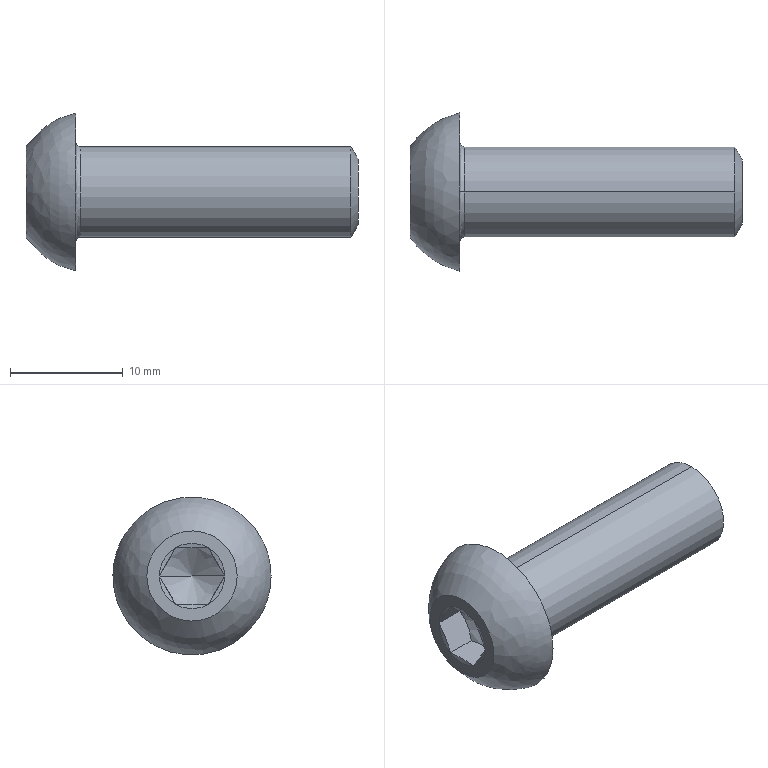Part | SolidWorks | features BaseBody 1 | 1 solid | 24 faces | box 29.4 x 14 x 14 mm | volume 1672 mm3 | cone 10 | plane 9 | spline 3 | cylinder 2 | commonest cylinder face diameters 8 x2
STEP:
#1=CARTESIAN_POINT('',(-24.6,0.,-4.));
#2=VERTEX_POINT('',#1);
#3=CARTESIAN_POINT('',(-24.6,0.,4.));
#4=VERTEX_POINT('',#3);
#5=CARTESIAN_POINT('',(-24.6,0.,0.));
#6=DIRECTION('',(1.,0.,0.));
#7=DIRECTION('',(0.,0.,1.));
#8=AXIS2_PLACEMENT_3D('',#5,#6,#7);
#9=CIRCLE('',#8,4.);
#10=EDGE_CURVE('',#2,#4,#9,.T.);
#11=ORIENTED_EDGE('',*,*,#10,.F.);
#12=CARTESIAN_POINT('',(-25.,0.,-4.4));
#13=VERTEX_POINT('',#12);
#14=CARTESIAN_POINT('',(-24.6,0.,-4.4));
#15=DIRECTION('',(0.,-1.,0.));
#16=DIRECTION('',(0.,0.,-1.));
#17=AXIS2_PLACEMENT_3D('',#14,#15,#16);
#18=CIRCLE('',#17,0.4);
#19=EDGE_CURVE('',#2,#13,#18,.T.);
#20=ORIENTED_EDGE('',*,*,#19,.T.);
#21=CARTESIAN_POINT('',(-25.,0.,4.4));
#22=VERTEX_POINT('',#21);
#23=CARTESIAN_POINT('',(-25.,0.,4.4));
#24=CARTESIAN_POINT('',(-25.,0.2798,4.4));
#25=CARTESIAN_POINT('',(-25.,0.6922,4.361));
#26=CARTESIAN_POINT('',(-25.,1.16,4.249));
#27=CARTESIAN_POINT('',(-25.,1.391,4.176));
#28=CARTESIAN_POINT('',(-25.,1.506,4.135));
#29=CARTESIAN_POINT('',(-25.,1.555,4.116));
#30=CARTESIAN_POINT('',(-25.,1.587,4.104));
#31=CARTESIAN_POINT('',(-25.,1.602,4.098));
#32=CARTESIAN_POINT('',(-25.,1.758,4.036));
#33=CARTESIAN_POINT('',(-25.,1.96,3.944));
#34=CARTESIAN_POINT('',(-25.,2.155,3.837));
#35=CARTESIAN_POINT('',(-25.,2.283,3.762));
#36=CARTESIAN_POINT('',(-25.,2.344,3.724));
#37=CARTESIAN_POINT('',(-25.,2.662,3.516));
#38=CARTESIAN_POINT('',(-25.,2.896,3.326));
#39=CARTESIAN_POINT('',(-25.,3.219,3.004));
#40=CARTESIAN_POINT('',(-25.,3.371,2.835));
#41=CARTESIAN_POINT('',(-25.,3.509,2.656));
#42=CARTESIAN_POINT('',(-25.,3.598,2.533));
#43=CARTESIAN_POINT('',(-25.,3.642,2.47));
#44=CARTESIAN_POINT('',(-25.,3.764,2.283));
#45=CARTESIAN_POINT('',(-25.,3.876,2.091));
#46=CARTESIAN_POINT('',(-25.,3.99,1.858));
#47=CARTESIAN_POINT('',(-25.,4.034,1.757));
#48=CARTESIAN_POINT('',(-25.,4.063,1.688));
#49=CARTESIAN_POINT('',(-25.,4.078,1.652));
#50=CARTESIAN_POINT('',(-25.,4.297,1.099));
#51=CARTESIAN_POINT('',(-25.,4.4,0.5599));
#52=CARTESIAN_POINT('',(-25.,4.4,-0.2799));
#53=CARTESIAN_POINT('',(-25.,4.361,-0.6923));
#54=CARTESIAN_POINT('',(-25.,4.249,-1.16));
#55=CARTESIAN_POINT('',(-25.,4.176,-1.391));
#56=CARTESIAN_POINT('',(-25.,4.135,-1.506));
#57=CARTESIAN_POINT('',(-25.,4.116,-1.555));
#58=CARTESIAN_POINT('',(-25.,4.104,-1.587));
#59=CARTESIAN_POINT('',(-25.,4.098,-1.602));
#60=CARTESIAN_POINT('',(-25.,4.036,-1.758));
#61=CARTESIAN_POINT('',(-25.,3.944,-1.96));
#62=CARTESIAN_POINT('',(-25.,3.837,-2.155));
#63=CARTESIAN_POINT('',(-25.,3.762,-2.283));
#64=CARTESIAN_POINT('',(-25.,3.724,-2.344));
#65=CARTESIAN_POINT('',(-25.,3.516,-2.662));
#66=CARTESIAN_POINT('',(-25.,3.326,-2.896));
#67=CARTESIAN_POINT('',(-25.,3.004,-3.219));
#68=CARTESIAN_POINT('',(-25.,2.835,-3.371));
#69=CARTESIAN_POINT('',(-25.,2.656,-3.509));
#70=CARTESIAN_POINT('',(-25.,2.533,-3.598));
#71=CARTESIAN_POINT('',(-25.,2.47,-3.642));
#72=CARTESIAN_POINT('',(-25.,2.283,-3.764));
#73=CARTESIAN_POINT('',(-25.,2.091,-3.876));
#74=CARTESIAN_POINT('',(-25.,1.858,-3.99));
#75=CARTESIAN_POINT('',(-25.,1.757,-4.034));
#76=CARTESIAN_POINT('',(-25.,1.688,-4.063));
#77=CARTESIAN_POINT('',(-25.,1.652,-4.078));
#78=CARTESIAN_POINT('',(-25.,1.099,-4.297));
#79=CARTESIAN_POINT('',(-25.,0.5593,-4.4));
#80=CARTESIAN_POINT('',(-25.,0.,-4.4));
#81=B_SPLINE_CURVE_WITH_KNOTS('',3,(#23,#24,#25,#26,#27,#28,#29,#30,#31,#32,#33,#34,#35,#36,#37,#38,#39,#40,#41,#42,#43,#44,#45,#46,#47,#48,#49,#50,#51,#52,#53,#54,#55,#56,#57,#58,#59,#60,#61,#62,#63,#64,#65,#66,#67,#68,#69,#70,#71,#72,#73,#74,#75,#76,#77,#78,#79,#80),.UNSPECIFIED.,.F.,.F.,(4,1,1,1,1,2,2,1,2,2,2,1,2,2,1,1,2,2,2,1,1,1,1,2,2,1,2,2,2,1,2,2,1,1,2,2,4),(0.,0.0625,0.09375,0.1094,0.1172,0.1211,0.125,0.1562,0.1719,0.1875,0.25,0.2812,0.2969,0.3125,0.3437,0.3594,0.3672,0.375,0.5,0.5625,0.5937,0.6094,0.6172,0.6211,0.625,0.6562,0.6719,0.6875,0.75,0.7812,0.7969,0.8125,0.8437,0.8594,0.8672,0.875,1.),.UNSPECIFIED.);
#82=EDGE_CURVE('',#22,#13,#81,.T.);
#83=ORIENTED_EDGE('',*,*,#82,.F.);
#84=CARTESIAN_POINT('',(-24.6,0.,4.4));
#85=DIRECTION('',(0.,1.,0.));
#86=DIRECTION('',(0.,0.,1.));
#87=AXIS2_PLACEMENT_3D('',#84,#85,#86);
#88=CIRCLE('',#87,0.4);
#89=EDGE_CURVE('',#4,#22,#88,.T.);
#90=ORIENTED_EDGE('',*,*,#89,.F.);
#91=EDGE_LOOP('',(#11,#20,#83,#90));
#92=FACE_OUTER_BOUND('',#91,.T.);
#93=CARTESIAN_POINT('',(-24.6,0.,4.));
#94=CARTESIAN_POINT('',(-24.6,8.,4.));
#95=CARTESIAN_POINT('',(-24.6,8.,-4.));
#96=CARTESIAN_POINT('',(-24.6,0.,-4.));
#97=CARTESIAN_POINT('',(-24.834,0.,4.));
#98=CARTESIAN_POINT('',(-24.834,8.,4.));
#99=CARTESIAN_POINT('',(-24.834,8.,-4.));
#100=CARTESIAN_POINT('',(-24.834,0.,-4.));
#101=CARTESIAN_POINT('',(-25.,0.,4.166));
#102=CARTESIAN_POINT('',(-25.,8.331,4.166));
#103=CARTESIAN_POINT('',(-25.,8.331,-4.166));
#104=CARTESIAN_POINT('',(-25.,0.,-4.166));
#105=CARTESIAN_POINT('',(-25.,0.,4.4));
#106=CARTESIAN_POINT('',(-25.,8.8,4.4));
#107=CARTESIAN_POINT('',(-25.,8.8,-4.4));
#108=CARTESIAN_POINT('',(-25.,0.,-4.4));
#109=(BOUNDED_SURFACE()B_SPLINE_SURFACE(3,3,((#93,#94,#95,#96),(#97,#98,#99,#100),(#101,#102,#103,#104),(#105,#106,#107,#108)),.UNSPECIFIED.,.F.,.F.,.F.)B_SPLINE_SURFACE_WITH_KNOTS((4,4),(4,4),(0.,1.),(0.,1.),.UNSPECIFIED.)GEOMETRIC_REPRESENTATION_ITEM()RATIONAL_B_SPLINE_SURFACE(((1.,0.3333,0.3333,1.),(0.8047,0.2682,0.2682,0.8047),(0.8047,0.2682,0.2682,0.8047),(1.,0.3333,0.3333,1.)))REPRESENTATION_ITEM('')SURFACE());
#110=ADVANCED_FACE('',(#92),#109,.F.);
#111=CARTESIAN_POINT('',(-0.625,0.,4.));
#112=VERTEX_POINT('',#111);
#113=CARTESIAN_POINT('',(-0.625,0.,-4.));
#114=VERTEX_POINT('',#113);
#115=CARTESIAN_POINT('',(-0.625,0.,0.));
#116=DIRECTION('',(-1.,0.,0.));
#117=DIRECTION('',(0.,0.,1.));
#118=AXIS2_PLACEMENT_3D('',#115,#116,#117);
#119=CIRCLE('',#118,4.);
#120=EDGE_CURVE('',#112,#114,#119,.T.);
#121=ORIENTED_EDGE('',*,*,#120,.T.);
#122=CARTESIAN_POINT('',(-29.4,0.,-4.));
#123=DIRECTION('',(-1.,0.,0.));
#124=VECTOR('',#123,1000.);
#125=LINE('',#122,#124);
#126=EDGE_CURVE('',#114,#2,#125,.T.);
#127=ORIENTED_EDGE('',*,*,#126,.T.);
#128=ORIENTED_EDGE('',*,*,#10,.T.);
#129=CARTESIAN_POINT('',(-29.4,0.,4.));
#130=DIRECTION('',(-1.,0.,0.));
#131=VECTOR('',#130,1000.);
#132=LINE('',#129,#131);
#133=EDGE_CURVE('',#112,#4,#132,.T.);
#134=ORIENTED_EDGE('',*,*,#133,.F.);
#135=EDGE_LOOP('',(#121,#127,#128,#134));
#136=FACE_OUTER_BOUND('',#135,.T.);
#137=CARTESIAN_POINT('',(-29.4,0.,0.));
#138=DIRECTION('',(-1.,0.,0.));
#139=DIRECTION('',(0.,0.,1.));
#140=AXIS2_PLACEMENT_3D('',#137,#138,#139);
#141=CYLINDRICAL_SURFACE('',#140,4.);
#142=ADVANCED_FACE('',(#136),#141,.T.);
#143=CARTESIAN_POINT('',(0.,0.,2.917));
#144=VERTEX_POINT('',#143);
#145=CARTESIAN_POINT('',(0.,0.,-2.917));
#146=VERTEX_POINT('',#145);
#147=CARTESIAN_POINT('',(0.,0.,0.));
#148=DIRECTION('',(-1.,0.,0.));
#149=DIRECTION('',(0.,0.,1.));
#150=AXIS2_PLACEMENT_3D('',#147,#148,#149);
#151=CIRCLE('',#150,2.917);
#152=EDGE_CURVE('',#144,#146,#151,.T.);
#153=ORIENTED_EDGE('',*,*,#152,.T.);
#154=CARTESIAN_POINT('',(-0.625,0.,-4.));
#155=DIRECTION('',(-0.5,0.,-0.866));
#156=VECTOR('',#155,1000.);
#157=LINE('',#154,#156);
#158=EDGE_CURVE('',#146,#114,#157,.T.);
#159=ORIENTED_EDGE('',*,*,#158,.T.);
#160=ORIENTED_EDGE('',*,*,#120,.F.);
#161=CARTESIAN_POINT('',(-0.625,0.,4.));
#162=DIRECTION('',(-0.5,0.,0.866));
#163=VECTOR('',#162,1000.);
#164=LINE('',#161,#163);
#165=EDGE_CURVE('',#144,#112,#164,.T.);
#166=ORIENTED_EDGE('',*,*,#165,.F.);
#167=EDGE_LOOP('',(#153,#159,#160,#166));
#168=FACE_OUTER_BOUND('',#167,.T.);
#169=CARTESIAN_POINT('',(-0.625,0.,0.));
#170=DIRECTION('',(-1.,0.,0.));
#171=DIRECTION('',(0.,0.,1.));
#172=AXIS2_PLACEMENT_3D('',#169,#170,#171);
#173=CONICAL_SURFACE('',#172,4.,1.047);
#174=ADVANCED_FACE('',(#168),#173,.T.);
#175=CARTESIAN_POINT('',(-25.,0.,0.));
#176=VERTEX_POINT('',#175);
#177=CARTESIAN_POINT('',(-26.8,-2.887,0.));
#178=VERTEX_POINT('',#177);
#179=CARTESIAN_POINT('',(-26.811,-2.904,0.));
#180=DIRECTION('',(-0.5291,-0.8486,0.));
#181=VECTOR('',#180,1000.);
#182=LINE('',#179,#181);
#183=EDGE_CURVE('',#176,#178,#182,.T.);
#184=ORIENTED_EDGE('',*,*,#183,.F.);
#185=CARTESIAN_POINT('',(-26.8,2.887,-0.000000014));
#186=VERTEX_POINT('',#185);
#187=CARTESIAN_POINT('',(-26.811,2.904,0.));
#188=DIRECTION('',(-0.5291,0.8486,0.));
#189=VECTOR('',#188,1000.);
#190=LINE('',#187,#189);
#191=EDGE_CURVE('',#176,#186,#190,.T.);
#192=ORIENTED_EDGE('',*,*,#191,.T.);
#193=CARTESIAN_POINT('',(-26.8,1.443,-2.5));
#194=VERTEX_POINT('',#193);
#195=CARTESIAN_POINT('',(-26.8,2.887,-0.000000014));
#196=CARTESIAN_POINT('',(-26.654,2.652,-0.4068));
#197=CARTESIAN_POINT('',(-26.559,2.413,-0.8206));
#198=CARTESIAN_POINT('',(-26.559,2.044,-1.46));
#199=CARTESIAN_POINT('',(-26.582,1.921,-1.673));
#200=CARTESIAN_POINT('',(-26.666,1.68,-2.09));
#201=CARTESIAN_POINT('',(-26.727,1.561,-2.296));
#202=CARTESIAN_POINT('',(-26.8,1.443,-2.5));
#203=B_SPLINE_CURVE_WITH_KNOTS('',3,(#195,#196,#197,#198,#199,#200,#201,#202),.UNSPECIFIED.,.F.,.F.,(4,2,2,4),(0.,0.00146,0.002189,0.002919),.UNSPECIFIED.);
#204=EDGE_CURVE('',#186,#194,#203,.T.);
#205=ORIENTED_EDGE('',*,*,#204,.T.);
#206=CARTESIAN_POINT('',(-26.8,-1.443,-2.5));
#207=VERTEX_POINT('',#206);
#208=CARTESIAN_POINT('',(-26.8,1.443,-2.5));
#209=CARTESIAN_POINT('',(-26.653,0.9733,-2.5));
#210=CARTESIAN_POINT('',(-26.559,0.4946,-2.5));
#211=CARTESIAN_POINT('',(-26.559,-0.4946,-2.5));
#212=CARTESIAN_POINT('',(-26.653,-0.9733,-2.5));
#213=CARTESIAN_POINT('',(-26.8,-1.443,-2.5));
#214=B_SPLINE_CURVE_WITH_KNOTS('',3,(#208,#209,#210,#211,#212,#213),.UNSPECIFIED.,.F.,.F.,(4,2,4),(-0.001463,0.,0.001463),.UNSPECIFIED.);
#215=EDGE_CURVE('',#194,#207,#214,.T.);
#216=ORIENTED_EDGE('',*,*,#215,.T.);
#217=CARTESIAN_POINT('',(-26.8,-1.443,-2.5));
#218=CARTESIAN_POINT('',(-26.654,-1.678,-2.093));
#219=CARTESIAN_POINT('',(-26.559,-1.917,-1.679));
#220=CARTESIAN_POINT('',(-26.559,-2.286,-1.04));
#221=CARTESIAN_POINT('',(-26.582,-2.409,-0.8268));
#222=CARTESIAN_POINT('',(-26.666,-2.65,-0.4095));
#223=CARTESIAN_POINT('',(-26.727,-2.769,-0.2038));
#224=CARTESIAN_POINT('',(-26.8,-2.887,0.));
#225=B_SPLINE_CURVE_WITH_KNOTS('',3,(#217,#218,#219,#220,#221,#222,#223,#224),.UNSPECIFIED.,.F.,.F.,(4,2,2,4),(0.,0.00146,0.002189,0.002919),.UNSPECIFIED.);
#226=EDGE_CURVE('',#207,#178,#225,.T.);
#227=ORIENTED_EDGE('',*,*,#226,.T.);
#228=EDGE_LOOP('',(#184,#192,#205,#216,#227));
#229=FACE_OUTER_BOUND('',#228,.T.);
#230=CARTESIAN_POINT('',(-26.811,0.,0.));
#231=DIRECTION('',(-1.,0.,0.));
#232=DIRECTION('',(0.,-1.,0.));
#233=AXIS2_PLACEMENT_3D('',#230,#231,#232);
#234=CONICAL_SURFACE('',#233,2.904,1.013);
#235=ADVANCED_FACE('',(#229),#234,.F.);
#236=ORIENTED_EDGE('',*,*,#126,.F.);
#237=CARTESIAN_POINT('',(-0.625,0.,0.));
#238=DIRECTION('',(-1.,0.,0.));
#239=DIRECTION('',(0.,0.,1.));
#240=AXIS2_PLACEMENT_3D('',#237,#238,#239);
#241=CIRCLE('',#240,4.);
#242=EDGE_CURVE('',#114,#112,#241,.T.);
#243=ORIENTED_EDGE('',*,*,#242,.T.);
#244=ORIENTED_EDGE('',*,*,#133,.T.);
#245=CARTESIAN_POINT('',(-24.6,0.,0.));
#246=DIRECTION('',(1.,0.,0.));
#247=DIRECTION('',(0.,0.,1.));
#248=AXIS2_PLACEMENT_3D('',#245,#246,#247);
#249=CIRCLE('',#248,4.);
#250=EDGE_CURVE('',#4,#2,#249,.T.);
#251=ORIENTED_EDGE('',*,*,#250,.T.);
#252=EDGE_LOOP('',(#236,#243,#244,#251));
#253=FACE_OUTER_BOUND('',#252,.T.);
#254=CARTESIAN_POINT('',(-29.4,0.,0.));
#255=DIRECTION('',(-1.,0.,0.));
#256=DIRECTION('',(0.,0.,1.));
#257=AXIS2_PLACEMENT_3D('',#254,#255,#256);
#258=CYLINDRICAL_SURFACE('',#257,4.);
#259=ADVANCED_FACE('',(#253),#258,.T.);
#260=ORIENTED_EDGE('',*,*,#19,.F.);
#261=ORIENTED_EDGE('',*,*,#250,.F.);
#262=ORIENTED_EDGE('',*,*,#89,.T.);
#263=CARTESIAN_POINT('',(-25.,0.,-4.4));
#264=CARTESIAN_POINT('',(-25.,-0.2798,-4.4));
#265=CARTESIAN_POINT('',(-25.,-0.6922,-4.361));
#266=CARTESIAN_POINT('',(-25.,-1.16,-4.249));
#267=CARTESIAN_POINT('',(-25.,-1.391,-4.176));
#268=CARTESIAN_POINT('',(-25.,-1.506,-4.135));
#269=CARTESIAN_POINT('',(-25.,-1.555,-4.116));
#270=CARTESIAN_POINT('',(-25.,-1.587,-4.104));
#271=CARTESIAN_POINT('',(-25.,-1.602,-4.098));
#272=CARTESIAN_POINT('',(-25.,-1.758,-4.036));
#273=CARTESIAN_POINT('',(-25.,-1.96,-3.944));
#274=CARTESIAN_POINT('',(-25.,-2.155,-3.837));
#275=CARTESIAN_POINT('',(-25.,-2.283,-3.762));
#276=CARTESIAN_POINT('',(-25.,-2.344,-3.724));
#277=CARTESIAN_POINT('',(-25.,-2.662,-3.516));
#278=CARTESIAN_POINT('',(-25.,-2.896,-3.326));
#279=CARTESIAN_POINT('',(-25.,-3.219,-3.004));
#280=CARTESIAN_POINT('',(-25.,-3.371,-2.835));
#281=CARTESIAN_POINT('',(-25.,-3.509,-2.656));
#282=CARTESIAN_POINT('',(-25.,-3.598,-2.533));
#283=CARTESIAN_POINT('',(-25.,-3.642,-2.47));
#284=CARTESIAN_POINT('',(-25.,-3.764,-2.283));
#285=CARTESIAN_POINT('',(-25.,-3.876,-2.091));
#286=CARTESIAN_POINT('',(-25.,-3.99,-1.858));
#287=CARTESIAN_POINT('',(-25.,-4.034,-1.757));
#288=CARTESIAN_POINT('',(-25.,-4.063,-1.688));
#289=CARTESIAN_POINT('',(-25.,-4.078,-1.652));
#290=CARTESIAN_POINT('',(-25.,-4.297,-1.099));
#291=CARTESIAN_POINT('',(-25.,-4.4,-0.5599));
#292=CARTESIAN_POINT('',(-25.,-4.4,0.2799));
#293=CARTESIAN_POINT('',(-25.,-4.361,0.6923));
#294=CARTESIAN_POINT('',(-25.,-4.249,1.16));
#295=CARTESIAN_POINT('',(-25.,-4.176,1.391));
#296=CARTESIAN_POINT('',(-25.,-4.135,1.506));
#297=CARTESIAN_POINT('',(-25.,-4.116,1.555));
#298=CARTESIAN_POINT('',(-25.,-4.104,1.587));
#299=CARTESIAN_POINT('',(-25.,-4.098,1.602));
#300=CARTESIAN_POINT('',(-25.,-4.036,1.758));
#301=CARTESIAN_POINT('',(-25.,-3.944,1.96));
#302=CARTESIAN_POINT('',(-25.,-3.837,2.155));
#303=CARTESIAN_POINT('',(-25.,-3.762,2.283));
#304=CARTESIAN_POINT('',(-25.,-3.724,2.344));
#305=CARTESIAN_POINT('',(-25.,-3.516,2.662));
#306=CARTESIAN_POINT('',(-25.,-3.326,2.896));
#307=CARTESIAN_POINT('',(-25.,-3.004,3.219));
#308=CARTESIAN_POINT('',(-25.,-2.835,3.371));
#309=CARTESIAN_POINT('',(-25.,-2.656,3.509));
#310=CARTESIAN_POINT('',(-25.,-2.533,3.598));
#311=CARTESIAN_POINT('',(-25.,-2.47,3.642));
#312=CARTESIAN_POINT('',(-25.,-2.283,3.764));
#313=CARTESIAN_POINT('',(-25.,-2.091,3.876));
#314=CARTESIAN_POINT('',(-25.,-1.858,3.99));
#315=CARTESIAN_POINT('',(-25.,-1.757,4.034));
#316=CARTESIAN_POINT('',(-25.,-1.688,4.063));
#317=CARTESIAN_POINT('',(-25.,-1.652,4.078));
#318=CARTESIAN_POINT('',(-25.,-1.099,4.297));
#319=CARTESIAN_POINT('',(-25.,-0.5593,4.4));
#320=CARTESIAN_POINT('',(-25.,0.,4.4));
#321=B_SPLINE_CURVE_WITH_KNOTS('',3,(#263,#264,#265,#266,#267,#268,#269,#270,#271,#272,#273,#274,#275,#276,#277,#278,#279,#280,#281,#282,#283,#284,#285,#286,#287,#288,#289,#290,#291,#292,#293,#294,#295,#296,#297,#298,#299,#300,#301,#302,#303,#304,#305,#306,#307,#308,#309,#310,#311,#312,#313,#314,#315,#316,#317,#318,#319,#320),.UNSPECIFIED.,.F.,.F.,(4,1,1,1,1,2,2,1,2,2,2,1,2,2,1,1,2,2,2,1,1,1,1,2,2,1,2,2,2,1,2,2,1,1,2,2,4),(0.,0.0625,0.09375,0.1094,0.1172,0.1211,0.125,0.1562,0.1719,0.1875,0.25,0.2812,0.2969,0.3125,0.3437,0.3594,0.3672,0.375,0.5,0.5625,0.5937,0.6094,0.6172,0.6211,0.625,0.6562,0.6719,0.6875,0.75,0.7812,0.7969,0.8125,0.8437,0.8594,0.8672,0.875,1.),.UNSPECIFIED.);
#322=EDGE_CURVE('',#13,#22,#321,.T.);
#323=ORIENTED_EDGE('',*,*,#322,.F.);
#324=EDGE_LOOP('',(#260,#261,#262,#323));
#325=FACE_OUTER_BOUND('',#324,.T.);
#326=CARTESIAN_POINT('',(-24.6,0.,-4.));
#327=CARTESIAN_POINT('',(-24.6,-8.,-4.));
#328=CARTESIAN_POINT('',(-24.6,-8.,4.));
#329=CARTESIAN_POINT('',(-24.6,0.,4.));
#330=CARTESIAN_POINT('',(-24.834,0.,-4.));
#331=CARTESIAN_POINT('',(-24.834,-8.,-4.));
#332=CARTESIAN_POINT('',(-24.834,-8.,4.));
#333=CARTESIAN_POINT('',(-24.834,0.,4.));
#334=CARTESIAN_POINT('',(-25.,0.,-4.166));
#335=CARTESIAN_POINT('',(-25.,-8.331,-4.166));
#336=CARTESIAN_POINT('',(-25.,-8.331,4.166));
#337=CARTESIAN_POINT('',(-25.,0.,4.166));
#338=CARTESIAN_POINT('',(-25.,0.,-4.4));
#339=CARTESIAN_POINT('',(-25.,-8.8,-4.4));
#340=CARTESIAN_POINT('',(-25.,-8.8,4.4));
#341=CARTESIAN_POINT('',(-25.,0.,4.4));
#342=(BOUNDED_SURFACE()B_SPLINE_SURFACE(3,3,((#326,#327,#328,#329),(#330,#331,#332,#333),(#334,#335,#336,#337),(#338,#339,#340,#341)),.UNSPECIFIED.,.F.,.F.,.F.)B_SPLINE_SURFACE_WITH_KNOTS((4,4),(4,4),(0.,1.),(0.,1.),.UNSPECIFIED.)GEOMETRIC_REPRESENTATION_ITEM()RATIONAL_B_SPLINE_SURFACE(((1.,0.3333,0.3333,1.),(0.8047,0.2682,0.2682,0.8047),(0.8047,0.2682,0.2682,0.8047),(1.,0.3333,0.3333,1.)))REPRESENTATION_ITEM('')SURFACE());
#343=ADVANCED_FACE('',(#325),#342,.F.);
#344=ORIENTED_EDGE('',*,*,#158,.F.);
#345=CARTESIAN_POINT('',(0.,0.,0.));
#346=DIRECTION('',(-1.,0.,0.));
#347=DIRECTION('',(0.,0.,1.));
#348=AXIS2_PLACEMENT_3D('',#345,#346,#347);
#349=CIRCLE('',#348,2.917);
#350=EDGE_CURVE('',#146,#144,#349,.T.);
#351=ORIENTED_EDGE('',*,*,#350,.T.);
#352=ORIENTED_EDGE('',*,*,#165,.T.);
#353=ORIENTED_EDGE('',*,*,#242,.F.);
#354=EDGE_LOOP('',(#344,#351,#352,#353));
#355=FACE_OUTER_BOUND('',#354,.T.);
#356=CARTESIAN_POINT('',(-0.625,0.,0.));
#357=DIRECTION('',(-1.,0.,0.));
#358=DIRECTION('',(0.,0.,1.));
#359=AXIS2_PLACEMENT_3D('',#356,#357,#358);
#360=CONICAL_SURFACE('',#359,4.,1.047);
#361=ADVANCED_FACE('',(#355),#360,.T.);
#362=ORIENTED_EDGE('',*,*,#322,.T.);
#363=ORIENTED_EDGE('',*,*,#82,.T.);
#364=EDGE_LOOP('',(#362,#363));
#365=FACE_BOUND('',#364,.T.);
#366=CARTESIAN_POINT('',(-25.,7.,0.));
#367=VERTEX_POINT('',#366);
#368=CARTESIAN_POINT('',(-25.,-7.,0.));
#369=VERTEX_POINT('',#368);
#370=CARTESIAN_POINT('',(-25.,7.,0.));
#371=CARTESIAN_POINT('',(-25.,7.,-0.4622));
#372=CARTESIAN_POINT('',(-25.,6.955,-0.9197));
#373=CARTESIAN_POINT('',(-25.,6.774,-1.825));
#374=CARTESIAN_POINT('',(-25.,6.64,-2.263));
#375=CARTESIAN_POINT('',(-25.,6.378,-2.895));
#376=CARTESIAN_POINT('',(-25.,6.28,-3.101));
#377=CARTESIAN_POINT('',(-25.,6.063,-3.506));
#378=CARTESIAN_POINT('',(-25.,5.944,-3.704));
#379=CARTESIAN_POINT('',(-25.,5.561,-4.277));
#380=CARTESIAN_POINT('',(-25.,5.271,-4.629));
#381=CARTESIAN_POINT('',(-25.,4.625,-5.274));
#382=CARTESIAN_POINT('',(-25.,4.264,-5.57));
#383=CARTESIAN_POINT('',(-25.,3.505,-6.077));
#384=CARTESIAN_POINT('',(-25.,3.103,-6.292));
#385=CARTESIAN_POINT('',(-25.,2.466,-6.555));
#386=CARTESIAN_POINT('',(-25.,2.248,-6.633));
#387=CARTESIAN_POINT('',(-25.,1.809,-6.766));
#388=CARTESIAN_POINT('',(-25.,1.587,-6.821));
#389=CARTESIAN_POINT('',(-25.,0.917,-6.955));
#390=CARTESIAN_POINT('',(-25.,0.4599,-7.));
#391=CARTESIAN_POINT('',(-25.,-0.4622,-7.));
#392=CARTESIAN_POINT('',(-25.,-0.9163,-6.955));
#393=CARTESIAN_POINT('',(-25.,-1.587,-6.821));
#394=CARTESIAN_POINT('',(-25.,-1.809,-6.766));
#395=CARTESIAN_POINT('',(-25.,-2.25,-6.633));
#396=CARTESIAN_POINT('',(-25.,-2.468,-6.555));
#397=CARTESIAN_POINT('',(-25.,-3.102,-6.292));
#398=CARTESIAN_POINT('',(-25.,-3.504,-6.077));
#399=CARTESIAN_POINT('',(-25.,-4.075,-5.696));
#400=CARTESIAN_POINT('',(-25.,-4.261,-5.558));
#401=CARTESIAN_POINT('',(-25.,-4.617,-5.266));
#402=CARTESIAN_POINT('',(-25.,-4.787,-5.113));
#403=CARTESIAN_POINT('',(-25.,-5.271,-4.629));
#404=CARTESIAN_POINT('',(-25.,-5.561,-4.277));
#405=CARTESIAN_POINT('',(-25.,-6.073,-3.511));
#406=CARTESIAN_POINT('',(-25.,-6.29,-3.105));
#407=CARTESIAN_POINT('',(-25.,-6.552,-2.474));
#408=CARTESIAN_POINT('',(-25.,-6.629,-2.259));
#409=CARTESIAN_POINT('',(-25.,-6.763,-1.821));
#410=CARTESIAN_POINT('',(-25.,-6.819,-1.596));
#411=CARTESIAN_POINT('',(-25.,-6.955,-0.919));
#412=CARTESIAN_POINT('',(-25.,-7.,-0.4622));
#413=CARTESIAN_POINT('',(-25.,-7.,0.));
#414=B_SPLINE_CURVE_WITH_KNOTS('',3,(#370,#371,#372,#373,#374,#375,#376,#377,#378,#379,#380,#381,#382,#383,#384,#385,#386,#387,#388,#389,#390,#391,#392,#393,#394,#395,#396,#397,#398,#399,#400,#401,#402,#403,#404,#405,#406,#407,#408,#409,#410,#411,#412,#413),.UNSPECIFIED.,.F.,.F.,(4,2,2,2,2,2,2,2,2,2,2,2,2,2,2,2,2,2,2,2,2,4),(0.,0.001379,0.002758,0.003448,0.004138,0.005517,0.006896,0.008275,0.008965,0.009654,0.01103,0.01241,0.0131,0.01379,0.01517,0.01586,0.01655,0.01793,0.01931,0.02,0.02069,0.02207),.UNSPECIFIED.);
#415=EDGE_CURVE('',#367,#369,#414,.T.);
#416=ORIENTED_EDGE('',*,*,#415,.F.);
#417=CARTESIAN_POINT('',(-25.,-7.,0.));
#418=CARTESIAN_POINT('',(-25.,-7.,0.4622));
#419=CARTESIAN_POINT('',(-25.,-6.955,0.9197));
#420=CARTESIAN_POINT('',(-25.,-6.774,1.825));
#421=CARTESIAN_POINT('',(-25.,-6.64,2.263));
#422=CARTESIAN_POINT('',(-25.,-6.378,2.895));
#423=CARTESIAN_POINT('',(-25.,-6.28,3.101));
#424=CARTESIAN_POINT('',(-25.,-6.063,3.506));
#425=CARTESIAN_POINT('',(-25.,-5.944,3.704));
#426=CARTESIAN_POINT('',(-25.,-5.561,4.277));
#427=CARTESIAN_POINT('',(-25.,-5.271,4.629));
#428=CARTESIAN_POINT('',(-25.,-4.625,5.274));
#429=CARTESIAN_POINT('',(-25.,-4.264,5.57));
#430=CARTESIAN_POINT('',(-25.,-3.505,6.077));
#431=CARTESIAN_POINT('',(-25.,-3.103,6.292));
#432=CARTESIAN_POINT('',(-25.,-2.466,6.555));
#433=CARTESIAN_POINT('',(-25.,-2.248,6.633));
#434=CARTESIAN_POINT('',(-25.,-1.809,6.766));
#435=CARTESIAN_POINT('',(-25.,-1.587,6.821));
#436=CARTESIAN_POINT('',(-25.,-0.917,6.955));
#437=CARTESIAN_POINT('',(-25.,-0.4599,7.));
#438=CARTESIAN_POINT('',(-25.,0.4622,7.));
#439=CARTESIAN_POINT('',(-25.,0.9163,6.955));
#440=CARTESIAN_POINT('',(-25.,1.587,6.821));
#441=CARTESIAN_POINT('',(-25.,1.809,6.766));
#442=CARTESIAN_POINT('',(-25.,2.25,6.633));
#443=CARTESIAN_POINT('',(-25.,2.468,6.555));
#444=CARTESIAN_POINT('',(-25.,3.102,6.292));
#445=CARTESIAN_POINT('',(-25.,3.504,6.077));
#446=CARTESIAN_POINT('',(-25.,4.075,5.696));
#447=CARTESIAN_POINT('',(-25.,4.261,5.558));
#448=CARTESIAN_POINT('',(-25.,4.617,5.266));
#449=CARTESIAN_POINT('',(-25.,4.787,5.113));
#450=CARTESIAN_POINT('',(-25.,5.271,4.629));
#451=CARTESIAN_POINT('',(-25.,5.561,4.277));
#452=CARTESIAN_POINT('',(-25.,6.073,3.511));
#453=CARTESIAN_POINT('',(-25.,6.29,3.105));
#454=CARTESIAN_POINT('',(-25.,6.552,2.474));
#455=CARTESIAN_POINT('',(-25.,6.629,2.259));
#456=CARTESIAN_POINT('',(-25.,6.763,1.821));
#457=CARTESIAN_POINT('',(-25.,6.819,1.596));
#458=CARTESIAN_POINT('',(-25.,6.955,0.919));
#459=CARTESIAN_POINT('',(-25.,7.,0.4622));
#460=CARTESIAN_POINT('',(-25.,7.,0.));
#461=B_SPLINE_CURVE_WITH_KNOTS('',3,(#417,#418,#419,#420,#421,#422,#423,#424,#425,#426,#427,#428,#429,#430,#431,#432,#433,#434,#435,#436,#437,#438,#439,#440,#441,#442,#443,#444,#445,#446,#447,#448,#449,#450,#451,#452,#453,#454,#455,#456,#457,#458,#459,#460),.UNSPECIFIED.,.F.,.F.,(4,2,2,2,2,2,2,2,2,2,2,2,2,2,2,2,2,2,2,2,2,4),(0.02207,0.02345,0.02483,0.02552,0.0262,0.02758,0.02896,0.03034,0.03103,0.03172,0.0331,0.03448,0.03517,0.03586,0.03724,0.03793,0.03862,0.04,0.04138,0.04207,0.04276,0.04413),.UNSPECIFIED.);
#462=EDGE_CURVE('',#369,#367,#461,.T.);
#463=ORIENTED_EDGE('',*,*,#462,.F.);
#464=EDGE_LOOP('',(#416,#463));
#465=FACE_OUTER_BOUND('',#464,.T.);
#466=CARTESIAN_POINT('',(-25.,4.4,0.));
#467=DIRECTION('',(-1.,0.,0.));
#468=DIRECTION('',(0.,0.,1.));
#469=AXIS2_PLACEMENT_3D('',#466,#467,#468);
#470=PLANE('',#469);
#471=ADVANCED_FACE('',(#365,#465),#470,.F.);
#472=ORIENTED_EDGE('',*,*,#152,.F.);
#473=ORIENTED_EDGE('',*,*,#350,.F.);
#474=EDGE_LOOP('',(#472,#473));
#475=FACE_OUTER_BOUND('',#474,.T.);
#476=CARTESIAN_POINT('',(0.,4.,0.));
#477=DIRECTION('',(-1.,0.,0.));
#478=DIRECTION('',(0.,0.,1.));
#479=AXIS2_PLACEMENT_3D('',#476,#477,#478);
#480=PLANE('',#479);
#481=ADVANCED_FACE('',(#475),#480,.F.);
#482=CARTESIAN_POINT('',(-29.4,-4.,0.));
#483=VERTEX_POINT('',#482);
#484=CARTESIAN_POINT('',(-29.4,4.,0.));
#485=VERTEX_POINT('',#484);
#486=CARTESIAN_POINT('',(-29.4,-4.,0.));
#487=CARTESIAN_POINT('',(-29.4,-4.,-0.2642));
#488=CARTESIAN_POINT('',(-29.4,-3.974,-0.5241));
#489=CARTESIAN_POINT('',(-29.4,-3.872,-1.035));
#490=CARTESIAN_POINT('',(-29.4,-3.796,-1.289));
#491=CARTESIAN_POINT('',(-29.4,-3.595,-1.774));
#492=CARTESIAN_POINT('',(-29.4,-3.472,-2.003));
#493=CARTESIAN_POINT('',(-29.4,-3.182,-2.438));
#494=CARTESIAN_POINT('',(-29.4,-3.013,-2.644));
#495=CARTESIAN_POINT('',(-29.4,-2.644,-3.013));
#496=CARTESIAN_POINT('',(-29.4,-2.443,-3.179));
#497=CARTESIAN_POINT('',(-29.4,-2.005,-3.471));
#498=CARTESIAN_POINT('',(-29.4,-1.773,-3.595));
#499=CARTESIAN_POINT('',(-29.4,-1.291,-3.795));
#500=CARTESIAN_POINT('',(-29.4,-1.039,-3.872));
#501=CARTESIAN_POINT('',(-29.4,-0.523,-3.974));
#502=CARTESIAN_POINT('',(-29.4,-0.2635,-4.));
#503=CARTESIAN_POINT('',(-29.4,0.2581,-4.));
#504=CARTESIAN_POINT('',(-29.4,0.5231,-3.974));
#505=CARTESIAN_POINT('',(-29.4,1.036,-3.872));
#506=CARTESIAN_POINT('',(-29.4,1.285,-3.797));
#507=CARTESIAN_POINT('',(-29.4,1.77,-3.597));
#508=CARTESIAN_POINT('',(-29.4,2.004,-3.472));
#509=CARTESIAN_POINT('',(-29.4,2.437,-3.182));
#510=CARTESIAN_POINT('',(-29.4,2.64,-3.017));
#511=CARTESIAN_POINT('',(-29.4,3.013,-2.644));
#512=CARTESIAN_POINT('',(-29.4,3.179,-2.442));
#513=CARTESIAN_POINT('',(-29.4,3.469,-2.009));
#514=CARTESIAN_POINT('',(-29.4,3.594,-1.775));
#515=CARTESIAN_POINT('',(-29.4,3.795,-1.29));
#516=CARTESIAN_POINT('',(-29.4,3.871,-1.041));
#517=CARTESIAN_POINT('',(-29.4,3.974,-0.5286));
#518=CARTESIAN_POINT('',(-29.4,4.,-0.2642));
#519=CARTESIAN_POINT('',(-29.4,4.,0.));
#520=B_SPLINE_CURVE_WITH_KNOTS('',3,(#486,#487,#488,#489,#490,#491,#492,#493,#494,#495,#496,#497,#498,#499,#500,#501,#502,#503,#504,#505,#506,#507,#508,#509,#510,#511,#512,#513,#514,#515,#516,#517,#518,#519),.UNSPECIFIED.,.F.,.F.,(4,2,2,2,2,2,2,2,2,2,2,2,2,2,2,2,4),(0.,0.0007815,0.001563,0.002344,0.003126,0.003907,0.004689,0.00547,0.006252,0.007033,0.007815,0.008596,0.009377,0.01016,0.01094,0.01172,0.0125),.UNSPECIFIED.);
#521=EDGE_CURVE('',#483,#485,#520,.T.);
#522=ORIENTED_EDGE('',*,*,#521,.T.);
#523=CARTESIAN_POINT('',(-29.4,4.,0.));
#524=CARTESIAN_POINT('',(-29.4,4.,0.2642));
#525=CARTESIAN_POINT('',(-29.4,3.974,0.5241));
#526=CARTESIAN_POINT('',(-29.4,3.872,1.035));
#527=CARTESIAN_POINT('',(-29.4,3.796,1.289));
#528=CARTESIAN_POINT('',(-29.4,3.595,1.774));
#529=CARTESIAN_POINT('',(-29.4,3.472,2.003));
#530=CARTESIAN_POINT('',(-29.4,3.182,2.438));
#531=CARTESIAN_POINT('',(-29.4,3.013,2.644));
#532=CARTESIAN_POINT('',(-29.4,2.644,3.013));
#533=CARTESIAN_POINT('',(-29.4,2.443,3.179));
#534=CARTESIAN_POINT('',(-29.4,2.005,3.471));
#535=CARTESIAN_POINT('',(-29.4,1.773,3.595));
#536=CARTESIAN_POINT('',(-29.4,1.291,3.795));
#537=CARTESIAN_POINT('',(-29.4,1.039,3.872));
#538=CARTESIAN_POINT('',(-29.4,0.523,3.974));
#539=CARTESIAN_POINT('',(-29.4,0.2635,4.));
#540=CARTESIAN_POINT('',(-29.4,-0.2581,4.));
#541=CARTESIAN_POINT('',(-29.4,-0.5231,3.974));
#542=CARTESIAN_POINT('',(-29.4,-1.036,3.872));
#543=CARTESIAN_POINT('',(-29.4,-1.285,3.797));
#544=CARTESIAN_POINT('',(-29.4,-1.77,3.597));
#545=CARTESIAN_POINT('',(-29.4,-2.004,3.472));
#546=CARTESIAN_POINT('',(-29.4,-2.437,3.182));
#547=CARTESIAN_POINT('',(-29.4,-2.64,3.017));
#548=CARTESIAN_POINT('',(-29.4,-3.013,2.644));
#549=CARTESIAN_POINT('',(-29.4,-3.179,2.442));
#550=CARTESIAN_POINT('',(-29.4,-3.469,2.009));
#551=CARTESIAN_POINT('',(-29.4,-3.594,1.775));
#552=CARTESIAN_POINT('',(-29.4,-3.795,1.29));
#553=CARTESIAN_POINT('',(-29.4,-3.871,1.041));
#554=CARTESIAN_POINT('',(-29.4,-3.974,0.5286));
#555=CARTESIAN_POINT('',(-29.4,-4.,0.2642));
#556=CARTESIAN_POINT('',(-29.4,-4.,0.));
#557=B_SPLINE_CURVE_WITH_KNOTS('',3,(#523,#524,#525,#526,#527,#528,#529,#530,#531,#532,#533,#534,#535,#536,#537,#538,#539,#540,#541,#542,#543,#544,#545,#546,#547,#548,#549,#550,#551,#552,#553,#554,#555,#556),.UNSPECIFIED.,.F.,.F.,(4,2,2,2,2,2,2,2,2,2,2,2,2,2,2,2,4),(0.0125,0.01328,0.01407,0.01485,0.01563,0.01641,0.01719,0.01797,0.01875,0.01954,0.02032,0.0211,0.02188,0.02266,0.02344,0.02423,0.02501),.UNSPECIFIED.);
#558=EDGE_CURVE('',#485,#483,#557,.T.);
#559=ORIENTED_EDGE('',*,*,#558,.T.);
#560=EDGE_LOOP('',(#522,#559));
#561=FACE_BOUND('',#560,.T.);
#562=ORIENTED_EDGE('',*,*,#415,.T.);
#563=ORIENTED_EDGE('',*,*,#462,.T.);
#564=EDGE_LOOP('',(#562,#563));
#565=FACE_OUTER_BOUND('',#564,.T.);
#566=CARTESIAN_POINT('',(-23.737,7.024,-1.407));
#567=CARTESIAN_POINT('',(-25.707,7.024,-1.005));
#568=CARTESIAN_POINT('',(-25.707,7.024,1.005));
#569=CARTESIAN_POINT('',(-23.737,7.024,1.407));
#570=CARTESIAN_POINT('',(-25.702,5.015,-11.035));
#571=CARTESIAN_POINT('',(-41.149,5.015,-7.883));
#572=CARTESIAN_POINT('',(-41.149,5.015,7.883));
#573=CARTESIAN_POINT('',(-25.702,5.015,11.035));
#574=CARTESIAN_POINT('',(-25.702,-5.015,-11.035));
#575=CARTESIAN_POINT('',(-41.149,-5.015,-7.883));
#576=CARTESIAN_POINT('',(-41.149,-5.015,7.883));
#577=CARTESIAN_POINT('',(-25.702,-5.015,11.035));
#578=CARTESIAN_POINT('',(-23.737,-7.024,-1.407));
#579=CARTESIAN_POINT('',(-25.707,-7.024,-1.005));
#580=CARTESIAN_POINT('',(-25.707,-7.024,1.005));
#581=CARTESIAN_POINT('',(-23.737,-7.024,1.407));
#582=(BOUNDED_SURFACE()B_SPLINE_SURFACE(3,3,((#566,#567,#568,#569),(#570,#571,#572,#573),(#574,#575,#576,#577),(#578,#579,#580,#581)),.UNSPECIFIED.,.F.,.F.,.F.)B_SPLINE_SURFACE_WITH_KNOTS((4,4),(4,4),(0.,1.),(0.,1.),.UNSPECIFIED.)GEOMETRIC_REPRESENTATION_ITEM()RATIONAL_B_SPLINE_SURFACE(((1.,0.4667,0.4667,1.),(0.4669,0.2179,0.2179,0.4669),(0.4669,0.2179,0.2179,0.4669),(1.,0.4667,0.4667,1.)))REPRESENTATION_ITEM('')SURFACE());
#583=ADVANCED_FACE('',(#561,#565),#582,.T.);
#584=CARTESIAN_POINT('',(-29.4,1.443,-2.5));
#585=VERTEX_POINT('',#584);
#586=CARTESIAN_POINT('',(-29.4,-1.443,-2.5));
#587=VERTEX_POINT('',#586);
#588=CARTESIAN_POINT('',(-29.4,0.,0.));
#589=DIRECTION('',(-1.,0.,0.));
#590=DIRECTION('',(0.,-1.,0.));
#591=AXIS2_PLACEMENT_3D('',#588,#589,#590);
#592=CIRCLE('',#591,2.887);
#593=EDGE_CURVE('',#585,#587,#592,.T.);
#594=ORIENTED_EDGE('',*,*,#593,.F.);
#595=CARTESIAN_POINT('',(-29.4,2.887,0.));
#596=VERTEX_POINT('',#595);
#597=CARTESIAN_POINT('',(-29.4,0.,0.));
#598=DIRECTION('',(-1.,0.,0.));
#599=DIRECTION('',(0.,-1.,0.));
#600=AXIS2_PLACEMENT_3D('',#597,#598,#599);
#601=CIRCLE('',#600,2.887);
#602=EDGE_CURVE('',#596,#585,#601,.T.);
#603=ORIENTED_EDGE('',*,*,#602,.F.);
#604=CARTESIAN_POINT('',(-29.4,1.443,2.5));
#605=VERTEX_POINT('',#604);
#606=CARTESIAN_POINT('',(-29.4,0.,0.));
#607=DIRECTION('',(-1.,0.,0.));
#608=DIRECTION('',(0.,-1.,0.));
#609=AXIS2_PLACEMENT_3D('',#606,#607,#608);
#610=CIRCLE('',#609,2.887);
#611=EDGE_CURVE('',#605,#596,#610,.T.);
#612=ORIENTED_EDGE('',*,*,#611,.F.);
#613=CARTESIAN_POINT('',(-29.4,-1.443,2.5));
#614=VERTEX_POINT('',#613);
#615=CARTESIAN_POINT('',(-29.4,0.,0.));
#616=DIRECTION('',(-1.,0.,0.));
#617=DIRECTION('',(0.,-1.,0.));
#618=AXIS2_PLACEMENT_3D('',#615,#616,#617);
#619=CIRCLE('',#618,2.887);
#620=EDGE_CURVE('',#614,#605,#619,.T.);
#621=ORIENTED_EDGE('',*,*,#620,.F.);
#622=CARTESIAN_POINT('',(-29.4,-2.887,0.));
#623=VERTEX_POINT('',#622);
#624=CARTESIAN_POINT('',(-29.4,0.,0.));
#625=DIRECTION('',(-1.,0.,0.));
#626=DIRECTION('',(0.,-1.,0.));
#627=AXIS2_PLACEMENT_3D('',#624,#625,#626);
#628=CIRCLE('',#627,2.887);
#629=EDGE_CURVE('',#623,#614,#628,.T.);
#630=ORIENTED_EDGE('',*,*,#629,.F.);
#631=CARTESIAN_POINT('',(-29.4,0.,0.));
#632=DIRECTION('',(-1.,0.,0.));
#633=DIRECTION('',(0.,-1.,0.));
#634=AXIS2_PLACEMENT_3D('',#631,#632,#633);
#635=CIRCLE('',#634,2.887);
#636=EDGE_CURVE('',#587,#623,#635,.T.);
#637=ORIENTED_EDGE('',*,*,#636,.F.);
#638=EDGE_LOOP('',(#594,#603,#612,#621,#630,#637));
#639=FACE_BOUND('',#638,.T.);
#640=ORIENTED_EDGE('',*,*,#521,.F.);
#641=ORIENTED_EDGE('',*,*,#558,.F.);
#642=EDGE_LOOP('',(#640,#641));
#643=FACE_OUTER_BOUND('',#642,.T.);
#644=CARTESIAN_POINT('',(-29.4,0.,0.));
#645=DIRECTION('',(1.,0.,0.));
#646=DIRECTION('',(0.,0.,-1.));
#647=AXIS2_PLACEMENT_3D('',#644,#645,#646);
#648=PLANE('',#647);
#649=ADVANCED_FACE('',(#639,#643),#648,.F.);
#650=ORIENTED_EDGE('',*,*,#636,.T.);
#651=CARTESIAN_POINT('',(-29.4,-1.443,-2.5));
#652=CARTESIAN_POINT('',(-29.34,-1.684,-2.083));
#653=CARTESIAN_POINT('',(-29.267,-2.165,-1.25));
#654=CARTESIAN_POINT('',(-29.34,-2.646,-0.4167));
#655=CARTESIAN_POINT('',(-29.4,-2.887,0.));
#656=B_SPLINE_CURVE_WITH_KNOTS('',3,(#651,#652,#653,#654,#655),.UNSPECIFIED.,.F.,.F.,(4,1,4),(0.,0.001443,0.002887),.UNSPECIFIED.);
#657=EDGE_CURVE('',#587,#623,#656,.T.);
#658=ORIENTED_EDGE('',*,*,#657,.F.);
#659=EDGE_LOOP('',(#650,#658));
#660=FACE_OUTER_BOUND('',#659,.T.);
#661=CARTESIAN_POINT('',(-29.4,0.,0.));
#662=DIRECTION('',(-1.,0.,0.));
#663=DIRECTION('',(0.,-1.,0.));
#664=AXIS2_PLACEMENT_3D('',#661,#662,#663);
#665=CONICAL_SURFACE('',#664,2.887,1.326);
#666=ADVANCED_FACE('',(#660),#665,.F.);
#667=ORIENTED_EDGE('',*,*,#593,.T.);
#668=CARTESIAN_POINT('',(-29.4,1.443,-2.5));
#669=CARTESIAN_POINT('',(-29.34,0.9623,-2.5));
#670=CARTESIAN_POINT('',(-29.267,0.,-2.5));
#671=CARTESIAN_POINT('',(-29.34,-0.9623,-2.5));
#672=CARTESIAN_POINT('',(-29.4,-1.443,-2.5));
#673=B_SPLINE_CURVE_WITH_KNOTS('',3,(#668,#669,#670,#671,#672),.UNSPECIFIED.,.F.,.F.,(4,1,4),(0.,0.001443,0.002887),.UNSPECIFIED.);
#674=EDGE_CURVE('',#585,#587,#673,.T.);
#675=ORIENTED_EDGE('',*,*,#674,.F.);
#676=EDGE_LOOP('',(#667,#675));
#677=FACE_OUTER_BOUND('',#676,.T.);
#678=CARTESIAN_POINT('',(-29.4,0.,0.));
#679=DIRECTION('',(-1.,0.,0.));
#680=DIRECTION('',(0.,-1.,0.));
#681=AXIS2_PLACEMENT_3D('',#678,#679,#680);
#682=CONICAL_SURFACE('',#681,2.887,1.326);
#683=ADVANCED_FACE('',(#677),#682,.F.);
#684=ORIENTED_EDGE('',*,*,#602,.T.);
#685=CARTESIAN_POINT('',(-29.4,2.887,0.));
#686=CARTESIAN_POINT('',(-29.34,2.646,-0.4167));
#687=CARTESIAN_POINT('',(-29.267,2.165,-1.25));
#688=CARTESIAN_POINT('',(-29.34,1.684,-2.083));
#689=CARTESIAN_POINT('',(-29.4,1.443,-2.5));
#690=B_SPLINE_CURVE_WITH_KNOTS('',3,(#685,#686,#687,#688,#689),.UNSPECIFIED.,.F.,.F.,(4,1,4),(0.,0.001443,0.002887),.UNSPECIFIED.);
#691=EDGE_CURVE('',#596,#585,#690,.T.);
#692=ORIENTED_EDGE('',*,*,#691,.F.);
#693=EDGE_LOOP('',(#684,#692));
#694=FACE_OUTER_BOUND('',#693,.T.);
#695=CARTESIAN_POINT('',(-29.4,0.,0.));
#696=DIRECTION('',(-1.,0.,0.));
#697=DIRECTION('',(0.,-1.,0.));
#698=AXIS2_PLACEMENT_3D('',#695,#696,#697);
#699=CONICAL_SURFACE('',#698,2.887,1.326);
#700=ADVANCED_FACE('',(#694),#699,.F.);
#701=ORIENTED_EDGE('',*,*,#611,.T.);
#702=CARTESIAN_POINT('',(-29.4,1.443,2.5));
#703=CARTESIAN_POINT('',(-29.34,1.684,2.083));
#704=CARTESIAN_POINT('',(-29.267,2.165,1.25));
#705=CARTESIAN_POINT('',(-29.34,2.646,0.4167));
#706=CARTESIAN_POINT('',(-29.4,2.887,0.));
#707=B_SPLINE_CURVE_WITH_KNOTS('',3,(#702,#703,#704,#705,#706),.UNSPECIFIED.,.F.,.F.,(4,1,4),(0.,0.001443,0.002887),.UNSPECIFIED.);
#708=EDGE_CURVE('',#605,#596,#707,.T.);
#709=ORIENTED_EDGE('',*,*,#708,.F.);
#710=EDGE_LOOP('',(#701,#709));
#711=FACE_OUTER_BOUND('',#710,.T.);
#712=CARTESIAN_POINT('',(-29.4,0.,0.));
#713=DIRECTION('',(-1.,0.,0.));
#714=DIRECTION('',(0.,-1.,0.));
#715=AXIS2_PLACEMENT_3D('',#712,#713,#714);
#716=CONICAL_SURFACE('',#715,2.887,1.326);
#717=ADVANCED_FACE('',(#711),#716,.F.);
#718=CARTESIAN_POINT('',(-29.4,1.443,2.5));
#719=CARTESIAN_POINT('',(-29.34,0.9641,2.5));
#720=CARTESIAN_POINT('',(-29.304,0.4833,2.5));
#721=CARTESIAN_POINT('',(-29.304,-0.4833,2.5));
#722=CARTESIAN_POINT('',(-29.34,-0.9641,2.5));
#723=CARTESIAN_POINT('',(-29.4,-1.443,2.5));
#724=B_SPLINE_CURVE_WITH_KNOTS('',3,(#718,#719,#720,#721,#722,#723),.UNSPECIFIED.,.F.,.F.,(4,2,4),(0.,0.001447,0.002893),.UNSPECIFIED.);
#725=EDGE_CURVE('',#605,#614,#724,.T.);
#726=ORIENTED_EDGE('',*,*,#725,.T.);
#727=ORIENTED_EDGE('',*,*,#620,.T.);
#728=EDGE_LOOP('',(#726,#727));
#729=FACE_OUTER_BOUND('',#728,.T.);
#730=CARTESIAN_POINT('',(-29.4,0.,0.));
#731=DIRECTION('',(-1.,0.,0.));
#732=DIRECTION('',(0.,-1.,0.));
#733=AXIS2_PLACEMENT_3D('',#730,#731,#732);
#734=CONICAL_SURFACE('',#733,2.887,1.326);
#735=ADVANCED_FACE('',(#729),#734,.F.);
#736=ORIENTED_EDGE('',*,*,#629,.T.);
#737=CARTESIAN_POINT('',(-29.4,-2.887,0.));
#738=CARTESIAN_POINT('',(-29.34,-2.646,0.4167));
#739=CARTESIAN_POINT('',(-29.267,-2.165,1.25));
#740=CARTESIAN_POINT('',(-29.34,-1.684,2.083));
#741=CARTESIAN_POINT('',(-29.4,-1.443,2.5));
#742=B_SPLINE_CURVE_WITH_KNOTS('',3,(#737,#738,#739,#740,#741),.UNSPECIFIED.,.F.,.F.,(4,1,4),(0.,0.001443,0.002887),.UNSPECIFIED.);
#743=EDGE_CURVE('',#623,#614,#742,.T.);
#744=ORIENTED_EDGE('',*,*,#743,.F.);
#745=EDGE_LOOP('',(#736,#744));
#746=FACE_OUTER_BOUND('',#745,.T.);
#747=CARTESIAN_POINT('',(-29.4,0.,0.));
#748=DIRECTION('',(-1.,0.,0.));
#749=DIRECTION('',(0.,-1.,0.));
#750=AXIS2_PLACEMENT_3D('',#747,#748,#749);
#751=CONICAL_SURFACE('',#750,2.887,1.326);
#752=ADVANCED_FACE('',(#746),#751,.F.);
#753=CARTESIAN_POINT('',(-25.,-2.887,0.));
#754=DIRECTION('',(-1.,0.,0.));
#755=VECTOR('',#754,1000.);
#756=LINE('',#753,#755);
#757=EDGE_CURVE('',#178,#623,#756,.T.);
#758=ORIENTED_EDGE('',*,*,#757,.F.);
#759=ORIENTED_EDGE('',*,*,#226,.F.);
#760=CARTESIAN_POINT('',(-25.,-1.443,-2.5));
#761=DIRECTION('',(1.,0.,0.));
#762=VECTOR('',#761,1000.);
#763=LINE('',#760,#762);
#764=EDGE_CURVE('',#587,#207,#763,.T.);
#765=ORIENTED_EDGE('',*,*,#764,.F.);
#766=ORIENTED_EDGE('',*,*,#657,.T.);
#767=EDGE_LOOP('',(#758,#759,#765,#766));
#768=FACE_OUTER_BOUND('',#767,.T.);
#769=CARTESIAN_POINT('',(-25.,-1.443,-2.5));
#770=DIRECTION('',(0.,-0.866,-0.5));
#771=DIRECTION('',(0.,0.5,-0.866));
#772=AXIS2_PLACEMENT_3D('',#769,#770,#771);
#773=PLANE('',#772);
#774=ADVANCED_FACE('',(#768),#773,.F.);
#775=ORIENTED_EDGE('',*,*,#764,.T.);
#776=ORIENTED_EDGE('',*,*,#215,.F.);
#777=CARTESIAN_POINT('',(-25.,1.443,-2.5));
#778=DIRECTION('',(1.,0.,0.));
#779=VECTOR('',#778,1000.);
#780=LINE('',#777,#779);
#781=EDGE_CURVE('',#585,#194,#780,.T.);
#782=ORIENTED_EDGE('',*,*,#781,.F.);
#783=ORIENTED_EDGE('',*,*,#674,.T.);
#784=EDGE_LOOP('',(#775,#776,#782,#783));
#785=FACE_OUTER_BOUND('',#784,.T.);
#786=CARTESIAN_POINT('',(-25.,1.443,-2.5));
#787=DIRECTION('',(0.,0.,-1.));
#788=DIRECTION('',(0.,1.,0.));
#789=AXIS2_PLACEMENT_3D('',#786,#787,#788);
#790=PLANE('',#789);
#791=ADVANCED_FACE('',(#785),#790,.F.);
#792=ORIENTED_EDGE('',*,*,#781,.T.);
#793=ORIENTED_EDGE('',*,*,#204,.F.);
#794=CARTESIAN_POINT('',(-25.,2.887,0.));
#795=DIRECTION('',(1.,0.,0.));
#796=VECTOR('',#795,1000.);
#797=LINE('',#794,#796);
#798=EDGE_CURVE('',#596,#186,#797,.T.);
#799=ORIENTED_EDGE('',*,*,#798,.F.);
#800=ORIENTED_EDGE('',*,*,#691,.T.);
#801=EDGE_LOOP('',(#792,#793,#799,#800));
#802=FACE_OUTER_BOUND('',#801,.T.);
#803=CARTESIAN_POINT('',(-25.,2.887,0.));
#804=DIRECTION('',(0.,0.866,-0.5));
#805=DIRECTION('',(0.,0.5,0.866));
#806=AXIS2_PLACEMENT_3D('',#803,#804,#805);
#807=PLANE('',#806);
#808=ADVANCED_FACE('',(#802),#807,.F.);
#809=ORIENTED_EDGE('',*,*,#798,.T.);
#810=CARTESIAN_POINT('',(-26.8,1.443,2.5));
#811=VERTEX_POINT('',#810);
#812=CARTESIAN_POINT('',(-26.8,1.443,2.5));
#813=CARTESIAN_POINT('',(-26.654,1.678,2.093));
#814=CARTESIAN_POINT('',(-26.559,1.917,1.679));
#815=CARTESIAN_POINT('',(-26.559,2.286,1.04));
#816=CARTESIAN_POINT('',(-26.582,2.409,0.8268));
#817=CARTESIAN_POINT('',(-26.666,2.65,0.4095));
#818=CARTESIAN_POINT('',(-26.727,2.769,0.2038));
#819=CARTESIAN_POINT('',(-26.8,2.887,-0.000000014));
#820=B_SPLINE_CURVE_WITH_KNOTS('',3,(#812,#813,#814,#815,#816,#817,#818,#819),.UNSPECIFIED.,.F.,.F.,(4,2,2,4),(0.,0.00146,0.002189,0.002919),.UNSPECIFIED.);
#821=EDGE_CURVE('',#811,#186,#820,.T.);
#822=ORIENTED_EDGE('',*,*,#821,.F.);
#823=CARTESIAN_POINT('',(-25.,1.443,2.5));
#824=DIRECTION('',(1.,0.,0.));
#825=VECTOR('',#824,1000.);
#826=LINE('',#823,#825);
#827=EDGE_CURVE('',#605,#811,#826,.T.);
#828=ORIENTED_EDGE('',*,*,#827,.F.);
#829=ORIENTED_EDGE('',*,*,#708,.T.);
#830=EDGE_LOOP('',(#809,#822,#828,#829));
#831=FACE_OUTER_BOUND('',#830,.T.);
#832=CARTESIAN_POINT('',(-25.,1.443,2.5));
#833=DIRECTION('',(0.,0.866,0.5));
#834=DIRECTION('',(0.,-0.5,0.866));
#835=AXIS2_PLACEMENT_3D('',#832,#833,#834);
#836=PLANE('',#835);
#837=ADVANCED_FACE('',(#831),#836,.F.);
#838=CARTESIAN_POINT('',(-26.8,-1.443,2.5));
#839=VERTEX_POINT('',#838);
#840=CARTESIAN_POINT('',(-25.,-1.443,2.5));
#841=DIRECTION('',(-1.,0.,0.));
#842=VECTOR('',#841,1000.);
#843=LINE('',#840,#842);
#844=EDGE_CURVE('',#839,#614,#843,.T.);
#845=ORIENTED_EDGE('',*,*,#844,.F.);
#846=CARTESIAN_POINT('',(-26.8,-2.887,0.));
#847=CARTESIAN_POINT('',(-26.654,-2.652,0.4068));
#848=CARTESIAN_POINT('',(-26.559,-2.413,0.8206));
#849=CARTESIAN_POINT('',(-26.559,-2.044,1.46));
#850=CARTESIAN_POINT('',(-26.582,-1.921,1.673));
#851=CARTESIAN_POINT('',(-26.666,-1.68,2.09));
#852=CARTESIAN_POINT('',(-26.727,-1.561,2.296));
#853=CARTESIAN_POINT('',(-26.8,-1.443,2.5));
#854=B_SPLINE_CURVE_WITH_KNOTS('',3,(#846,#847,#848,#849,#850,#851,#852,#853),.UNSPECIFIED.,.F.,.F.,(4,2,2,4),(0.,0.00146,0.002189,0.002919),.UNSPECIFIED.);
#855=EDGE_CURVE('',#178,#839,#854,.T.);
#856=ORIENTED_EDGE('',*,*,#855,.F.);
#857=ORIENTED_EDGE('',*,*,#757,.T.);
#858=ORIENTED_EDGE('',*,*,#743,.T.);
#859=EDGE_LOOP('',(#845,#856,#857,#858));
#860=FACE_OUTER_BOUND('',#859,.T.);
#861=CARTESIAN_POINT('',(-25.,-2.887,0.));
#862=DIRECTION('',(0.,-0.866,0.5));
#863=DIRECTION('',(0.,-0.5,-0.866));
#864=AXIS2_PLACEMENT_3D('',#861,#862,#863);
#865=PLANE('',#864);
#866=ADVANCED_FACE('',(#860),#865,.F.);
#867=ORIENTED_EDGE('',*,*,#191,.F.);
#868=ORIENTED_EDGE('',*,*,#183,.T.);
#869=ORIENTED_EDGE('',*,*,#855,.T.);
#870=CARTESIAN_POINT('',(-26.8,1.443,2.5));
#871=CARTESIAN_POINT('',(-26.653,0.9733,2.5));
#872=CARTESIAN_POINT('',(-26.559,0.4946,2.5));
#873=CARTESIAN_POINT('',(-26.559,-0.4946,2.5));
#874=CARTESIAN_POINT('',(-26.653,-0.9733,2.5));
#875=CARTESIAN_POINT('',(-26.8,-1.443,2.5));
#876=B_SPLINE_CURVE_WITH_KNOTS('',3,(#870,#871,#872,#873,#874,#875),.UNSPECIFIED.,.F.,.F.,(4,2,4),(-0.001463,0.,0.001463),.UNSPECIFIED.);
#877=EDGE_CURVE('',#811,#839,#876,.T.);
#878=ORIENTED_EDGE('',*,*,#877,.F.);
#879=ORIENTED_EDGE('',*,*,#821,.T.);
#880=EDGE_LOOP('',(#867,#868,#869,#878,#879));
#881=FACE_OUTER_BOUND('',#880,.T.);
#882=CARTESIAN_POINT('',(-26.811,0.,0.));
#883=DIRECTION('',(-1.,0.,0.));
#884=DIRECTION('',(0.,-1.,0.));
#885=AXIS2_PLACEMENT_3D('',#882,#883,#884);
#886=CONICAL_SURFACE('',#885,2.904,1.013);
#887=ADVANCED_FACE('',(#881),#886,.F.);
#888=ORIENTED_EDGE('',*,*,#827,.T.);
#889=ORIENTED_EDGE('',*,*,#877,.T.);
#890=ORIENTED_EDGE('',*,*,#844,.T.);
#891=ORIENTED_EDGE('',*,*,#725,.F.);
#892=EDGE_LOOP('',(#888,#889,#890,#891));
#893=FACE_OUTER_BOUND('',#892,.T.);
#894=CARTESIAN_POINT('',(-25.,-1.443,2.5));
#895=DIRECTION('',(0.,0.,1.));
#896=DIRECTION('',(1.,0.,0.));
#897=AXIS2_PLACEMENT_3D('',#894,#895,#896);
#898=PLANE('',#897);
#899=ADVANCED_FACE('',(#893),#898,.F.);
#900=CLOSED_SHELL('',(#110,#142,#174,#235,#259,#343,#361,#471,#481,#583,#649,#666,#683,#700,#717,#735,#752,#774,#791,#808,#837,#866,#887,#899));
#901=MANIFOLD_SOLID_BREP('',#900);
#902=CARTESIAN_POINT('',(0.,0.,0.));
#903=DIRECTION('',(0.,0.,1.));
#904=DIRECTION('',(1.,0.,0.));
#905=AXIS2_PLACEMENT_3D('',#902,#903,#904);
#906=(LENGTH_UNIT()NAMED_UNIT(*)SI_UNIT(.MILLI.,.METRE.));
#907=UNCERTAINTY_MEASURE_WITH_UNIT(LENGTH_MEASURE(0.00001),#906,'','');
#908=(NAMED_UNIT(*)PLANE_ANGLE_UNIT()SI_UNIT($,.RADIAN.));
#909=(NAMED_UNIT(*)SI_UNIT($,.STERADIAN.)SOLID_ANGLE_UNIT());
#910=(GEOMETRIC_REPRESENTATION_CONTEXT(3)GLOBAL_UNCERTAINTY_ASSIGNED_CONTEXT((#907))GLOBAL_UNIT_ASSIGNED_CONTEXT((#906,#908,#909))REPRESENTATION_CONTEXT('',''));
#911=ADVANCED_BREP_SHAPE_REPRESENTATION('',(#901,#905),#910);